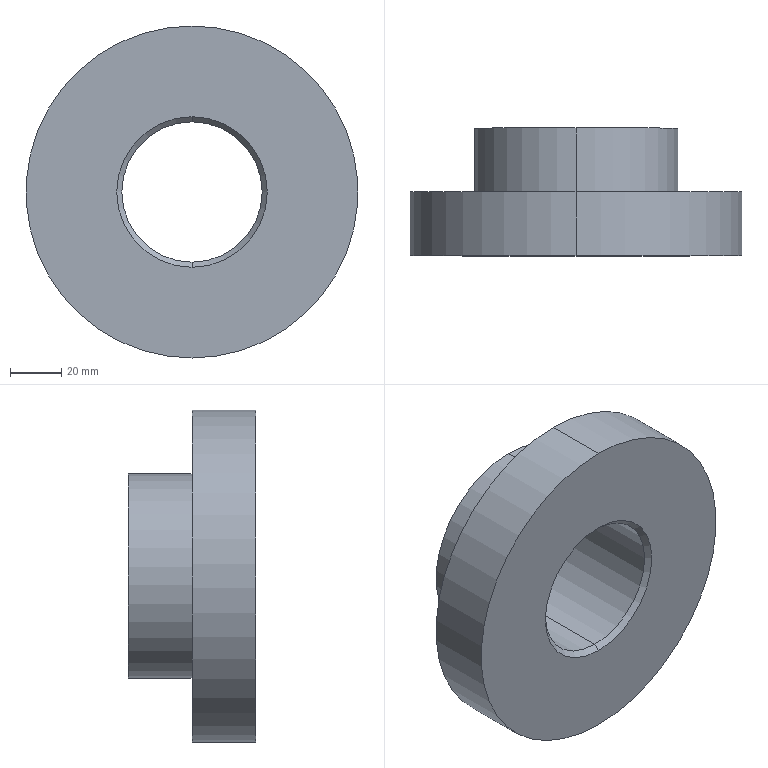Part | SolidWorks | features Revolution 1 | 1 solid | 11 faces | box 130 x 50 x 130 mm | volume 338349 mm3 | cylinder 6 | plane 3 | cone 2 | commonest cylinder face diameters 55 x2 80 x2 130 x2
STEP:
#1=CARTESIAN_POINT('',(0.,2.,27.5));
#2=VERTEX_POINT('',#1);
#3=CARTESIAN_POINT('',(0.,2.,-27.5));
#4=VERTEX_POINT('',#3);
#5=CARTESIAN_POINT('',(0.,2.,0.));
#6=DIRECTION('',(0.,-1.,0.));
#7=DIRECTION('',(0.,0.,-1.));
#8=AXIS2_PLACEMENT_3D('',#5,#6,#7);
#9=CIRCLE('',#8,27.5);
#10=EDGE_CURVE('',#2,#4,#9,.T.);
#11=ORIENTED_EDGE('',*,*,#10,.F.);
#12=CARTESIAN_POINT('',(0.,0.,29.5));
#13=VERTEX_POINT('',#12);
#14=CARTESIAN_POINT('',(0.,0.,29.5));
#15=DIRECTION('',(0.,-0.7071,0.7071));
#16=VECTOR('',#15,1000.);
#17=LINE('',#14,#16);
#18=EDGE_CURVE('',#2,#13,#17,.T.);
#19=ORIENTED_EDGE('',*,*,#18,.T.);
#20=CARTESIAN_POINT('',(0.,0.,-29.5));
#21=VERTEX_POINT('',#20);
#22=CARTESIAN_POINT('',(0.,0.,0.));
#23=DIRECTION('',(0.,-1.,0.));
#24=DIRECTION('',(0.,0.,-1.));
#25=AXIS2_PLACEMENT_3D('',#22,#23,#24);
#26=CIRCLE('',#25,29.5);
#27=EDGE_CURVE('',#13,#21,#26,.T.);
#28=ORIENTED_EDGE('',*,*,#27,.T.);
#29=CARTESIAN_POINT('',(0.,0.,-29.5));
#30=DIRECTION('',(0.,-0.7071,-0.7071));
#31=VECTOR('',#30,1000.);
#32=LINE('',#29,#31);
#33=EDGE_CURVE('',#4,#21,#32,.T.);
#34=ORIENTED_EDGE('',*,*,#33,.F.);
#35=EDGE_LOOP('',(#11,#19,#28,#34));
#36=FACE_OUTER_BOUND('',#35,.T.);
#37=CARTESIAN_POINT('',(0.,0.,0.));
#38=DIRECTION('',(0.,-1.,0.));
#39=DIRECTION('',(0.,0.,-1.));
#40=AXIS2_PLACEMENT_3D('',#37,#38,#39);
#41=CONICAL_SURFACE('',#40,29.5,0.7854);
#42=ADVANCED_FACE('',(#36),#41,.F.);
#43=CARTESIAN_POINT('',(0.,50.,27.5));
#44=VERTEX_POINT('',#43);
#45=CARTESIAN_POINT('',(0.,50.,-27.5));
#46=VERTEX_POINT('',#45);
#47=CARTESIAN_POINT('',(0.,50.,0.));
#48=DIRECTION('',(0.,-1.,0.));
#49=DIRECTION('',(0.,0.,-1.));
#50=AXIS2_PLACEMENT_3D('',#47,#48,#49);
#51=CIRCLE('',#50,27.5);
#52=EDGE_CURVE('',#44,#46,#51,.T.);
#53=ORIENTED_EDGE('',*,*,#52,.F.);
#54=CARTESIAN_POINT('',(0.,0.,27.5));
#55=DIRECTION('',(0.,-1.,0.));
#56=VECTOR('',#55,1000.);
#57=LINE('',#54,#56);
#58=EDGE_CURVE('',#44,#2,#57,.T.);
#59=ORIENTED_EDGE('',*,*,#58,.T.);
#60=ORIENTED_EDGE('',*,*,#10,.T.);
#61=CARTESIAN_POINT('',(0.,0.,-27.5));
#62=DIRECTION('',(0.,-1.,0.));
#63=VECTOR('',#62,1000.);
#64=LINE('',#61,#63);
#65=EDGE_CURVE('',#46,#4,#64,.T.);
#66=ORIENTED_EDGE('',*,*,#65,.F.);
#67=EDGE_LOOP('',(#53,#59,#60,#66));
#68=FACE_OUTER_BOUND('',#67,.T.);
#69=CARTESIAN_POINT('',(0.,0.,0.));
#70=DIRECTION('',(0.,-1.,0.));
#71=DIRECTION('',(0.,0.,-1.));
#72=AXIS2_PLACEMENT_3D('',#69,#70,#71);
#73=CYLINDRICAL_SURFACE('',#72,27.5);
#74=ADVANCED_FACE('',(#68),#73,.F.);
#75=CARTESIAN_POINT('',(0.,50.,-40.));
#76=VERTEX_POINT('',#75);
#77=CARTESIAN_POINT('',(0.,50.,40.));
#78=VERTEX_POINT('',#77);
#79=CARTESIAN_POINT('',(0.,50.,0.));
#80=DIRECTION('',(0.,-1.,0.));
#81=DIRECTION('',(0.,0.,-1.));
#82=AXIS2_PLACEMENT_3D('',#79,#80,#81);
#83=CIRCLE('',#82,40.);
#84=EDGE_CURVE('',#76,#78,#83,.T.);
#85=ORIENTED_EDGE('',*,*,#84,.T.);
#86=CARTESIAN_POINT('',(0.,25.,40.));
#87=VERTEX_POINT('',#86);
#88=CARTESIAN_POINT('',(0.,0.,40.));
#89=DIRECTION('',(0.,-1.,0.));
#90=VECTOR('',#89,1000.);
#91=LINE('',#88,#90);
#92=EDGE_CURVE('',#78,#87,#91,.T.);
#93=ORIENTED_EDGE('',*,*,#92,.T.);
#94=CARTESIAN_POINT('',(0.,25.,-40.));
#95=VERTEX_POINT('',#94);
#96=CARTESIAN_POINT('',(0.,25.,0.));
#97=DIRECTION('',(0.,-1.,0.));
#98=DIRECTION('',(0.,0.,-1.));
#99=AXIS2_PLACEMENT_3D('',#96,#97,#98);
#100=CIRCLE('',#99,40.);
#101=EDGE_CURVE('',#95,#87,#100,.T.);
#102=ORIENTED_EDGE('',*,*,#101,.F.);
#103=CARTESIAN_POINT('',(0.,0.,-40.));
#104=DIRECTION('',(0.,-1.,0.));
#105=VECTOR('',#104,1000.);
#106=LINE('',#103,#105);
#107=EDGE_CURVE('',#76,#95,#106,.T.);
#108=ORIENTED_EDGE('',*,*,#107,.F.);
#109=EDGE_LOOP('',(#85,#93,#102,#108));
#110=FACE_OUTER_BOUND('',#109,.T.);
#111=CARTESIAN_POINT('',(0.,0.,0.));
#112=DIRECTION('',(0.,-1.,0.));
#113=DIRECTION('',(0.,0.,-1.));
#114=AXIS2_PLACEMENT_3D('',#111,#112,#113);
#115=CYLINDRICAL_SURFACE('',#114,40.);
#116=ADVANCED_FACE('',(#110),#115,.T.);
#117=CARTESIAN_POINT('',(0.,25.,-65.));
#118=VERTEX_POINT('',#117);
#119=CARTESIAN_POINT('',(0.,25.,65.));
#120=VERTEX_POINT('',#119);
#121=CARTESIAN_POINT('',(0.,25.,0.));
#122=DIRECTION('',(0.,-1.,0.));
#123=DIRECTION('',(0.,0.,-1.));
#124=AXIS2_PLACEMENT_3D('',#121,#122,#123);
#125=CIRCLE('',#124,65.);
#126=EDGE_CURVE('',#118,#120,#125,.T.);
#127=ORIENTED_EDGE('',*,*,#126,.T.);
#128=CARTESIAN_POINT('',(0.,0.,65.));
#129=VERTEX_POINT('',#128);
#130=CARTESIAN_POINT('',(0.,0.,65.));
#131=DIRECTION('',(0.,-1.,0.));
#132=VECTOR('',#131,1000.);
#133=LINE('',#130,#132);
#134=EDGE_CURVE('',#120,#129,#133,.T.);
#135=ORIENTED_EDGE('',*,*,#134,.T.);
#136=CARTESIAN_POINT('',(0.,0.,-65.));
#137=VERTEX_POINT('',#136);
#138=CARTESIAN_POINT('',(0.,0.,0.));
#139=DIRECTION('',(0.,-1.,0.));
#140=DIRECTION('',(0.,0.,-1.));
#141=AXIS2_PLACEMENT_3D('',#138,#139,#140);
#142=CIRCLE('',#141,65.);
#143=EDGE_CURVE('',#137,#129,#142,.T.);
#144=ORIENTED_EDGE('',*,*,#143,.F.);
#145=CARTESIAN_POINT('',(0.,0.,-65.));
#146=DIRECTION('',(0.,-1.,0.));
#147=VECTOR('',#146,1000.);
#148=LINE('',#145,#147);
#149=EDGE_CURVE('',#118,#137,#148,.T.);
#150=ORIENTED_EDGE('',*,*,#149,.F.);
#151=EDGE_LOOP('',(#127,#135,#144,#150));
#152=FACE_OUTER_BOUND('',#151,.T.);
#153=CARTESIAN_POINT('',(0.,0.,0.));
#154=DIRECTION('',(0.,-1.,0.));
#155=DIRECTION('',(0.,0.,-1.));
#156=AXIS2_PLACEMENT_3D('',#153,#154,#155);
#157=CYLINDRICAL_SURFACE('',#156,65.);
#158=ADVANCED_FACE('',(#152),#157,.T.);
#159=ORIENTED_EDGE('',*,*,#134,.F.);
#160=CARTESIAN_POINT('',(0.,25.,0.));
#161=DIRECTION('',(0.,-1.,0.));
#162=DIRECTION('',(0.,0.,-1.));
#163=AXIS2_PLACEMENT_3D('',#160,#161,#162);
#164=CIRCLE('',#163,65.);
#165=EDGE_CURVE('',#120,#118,#164,.T.);
#166=ORIENTED_EDGE('',*,*,#165,.T.);
#167=ORIENTED_EDGE('',*,*,#149,.T.);
#168=CARTESIAN_POINT('',(0.,0.,0.));
#169=DIRECTION('',(0.,-1.,0.));
#170=DIRECTION('',(0.,0.,-1.));
#171=AXIS2_PLACEMENT_3D('',#168,#169,#170);
#172=CIRCLE('',#171,65.);
#173=EDGE_CURVE('',#129,#137,#172,.T.);
#174=ORIENTED_EDGE('',*,*,#173,.F.);
#175=EDGE_LOOP('',(#159,#166,#167,#174));
#176=FACE_OUTER_BOUND('',#175,.T.);
#177=CARTESIAN_POINT('',(0.,0.,0.));
#178=DIRECTION('',(0.,-1.,0.));
#179=DIRECTION('',(0.,0.,-1.));
#180=AXIS2_PLACEMENT_3D('',#177,#178,#179);
#181=CYLINDRICAL_SURFACE('',#180,65.);
#182=ADVANCED_FACE('',(#176),#181,.T.);
#183=ORIENTED_EDGE('',*,*,#126,.F.);
#184=ORIENTED_EDGE('',*,*,#165,.F.);
#185=EDGE_LOOP('',(#183,#184));
#186=FACE_OUTER_BOUND('',#185,.T.);
#187=ORIENTED_EDGE('',*,*,#101,.T.);
#188=CARTESIAN_POINT('',(0.,25.,0.));
#189=DIRECTION('',(0.,-1.,0.));
#190=DIRECTION('',(0.,0.,-1.));
#191=AXIS2_PLACEMENT_3D('',#188,#189,#190);
#192=CIRCLE('',#191,40.);
#193=EDGE_CURVE('',#87,#95,#192,.T.);
#194=ORIENTED_EDGE('',*,*,#193,.T.);
#195=EDGE_LOOP('',(#187,#194));
#196=FACE_BOUND('',#195,.T.);
#197=CARTESIAN_POINT('',(-65.,25.,0.));
#198=DIRECTION('',(0.,-1.,0.));
#199=DIRECTION('',(0.,0.,-1.));
#200=AXIS2_PLACEMENT_3D('',#197,#198,#199);
#201=PLANE('',#200);
#202=ADVANCED_FACE('',(#186,#196),#201,.F.);
#203=ORIENTED_EDGE('',*,*,#92,.F.);
#204=CARTESIAN_POINT('',(0.,50.,0.));
#205=DIRECTION('',(0.,-1.,0.));
#206=DIRECTION('',(0.,0.,-1.));
#207=AXIS2_PLACEMENT_3D('',#204,#205,#206);
#208=CIRCLE('',#207,40.);
#209=EDGE_CURVE('',#78,#76,#208,.T.);
#210=ORIENTED_EDGE('',*,*,#209,.T.);
#211=ORIENTED_EDGE('',*,*,#107,.T.);
#212=ORIENTED_EDGE('',*,*,#193,.F.);
#213=EDGE_LOOP('',(#203,#210,#211,#212));
#214=FACE_OUTER_BOUND('',#213,.T.);
#215=CARTESIAN_POINT('',(0.,0.,0.));
#216=DIRECTION('',(0.,-1.,0.));
#217=DIRECTION('',(0.,0.,-1.));
#218=AXIS2_PLACEMENT_3D('',#215,#216,#217);
#219=CYLINDRICAL_SURFACE('',#218,40.);
#220=ADVANCED_FACE('',(#214),#219,.T.);
#221=ORIENTED_EDGE('',*,*,#84,.F.);
#222=ORIENTED_EDGE('',*,*,#209,.F.);
#223=EDGE_LOOP('',(#221,#222));
#224=FACE_OUTER_BOUND('',#223,.T.);
#225=CARTESIAN_POINT('',(0.,50.,0.));
#226=DIRECTION('',(0.,-1.,0.));
#227=DIRECTION('',(0.,0.,-1.));
#228=AXIS2_PLACEMENT_3D('',#225,#226,#227);
#229=CIRCLE('',#228,27.5);
#230=EDGE_CURVE('',#46,#44,#229,.T.);
#231=ORIENTED_EDGE('',*,*,#230,.T.);
#232=ORIENTED_EDGE('',*,*,#52,.T.);
#233=EDGE_LOOP('',(#231,#232));
#234=FACE_BOUND('',#233,.T.);
#235=CARTESIAN_POINT('',(-40.,50.,0.));
#236=DIRECTION('',(0.,-1.,0.));
#237=DIRECTION('',(0.,0.,-1.));
#238=AXIS2_PLACEMENT_3D('',#235,#236,#237);
#239=PLANE('',#238);
#240=ADVANCED_FACE('',(#224,#234),#239,.F.);
#241=ORIENTED_EDGE('',*,*,#58,.F.);
#242=ORIENTED_EDGE('',*,*,#230,.F.);
#243=ORIENTED_EDGE('',*,*,#65,.T.);
#244=CARTESIAN_POINT('',(0.,2.,0.));
#245=DIRECTION('',(0.,-1.,0.));
#246=DIRECTION('',(0.,0.,-1.));
#247=AXIS2_PLACEMENT_3D('',#244,#245,#246);
#248=CIRCLE('',#247,27.5);
#249=EDGE_CURVE('',#4,#2,#248,.T.);
#250=ORIENTED_EDGE('',*,*,#249,.T.);
#251=EDGE_LOOP('',(#241,#242,#243,#250));
#252=FACE_OUTER_BOUND('',#251,.T.);
#253=CARTESIAN_POINT('',(0.,0.,0.));
#254=DIRECTION('',(0.,-1.,0.));
#255=DIRECTION('',(0.,0.,-1.));
#256=AXIS2_PLACEMENT_3D('',#253,#254,#255);
#257=CYLINDRICAL_SURFACE('',#256,27.5);
#258=ADVANCED_FACE('',(#252),#257,.F.);
#259=ORIENTED_EDGE('',*,*,#18,.F.);
#260=ORIENTED_EDGE('',*,*,#249,.F.);
#261=ORIENTED_EDGE('',*,*,#33,.T.);
#262=CARTESIAN_POINT('',(0.,0.,0.));
#263=DIRECTION('',(0.,-1.,0.));
#264=DIRECTION('',(0.,0.,-1.));
#265=AXIS2_PLACEMENT_3D('',#262,#263,#264);
#266=CIRCLE('',#265,29.5);
#267=EDGE_CURVE('',#21,#13,#266,.T.);
#268=ORIENTED_EDGE('',*,*,#267,.T.);
#269=EDGE_LOOP('',(#259,#260,#261,#268));
#270=FACE_OUTER_BOUND('',#269,.T.);
#271=CARTESIAN_POINT('',(0.,0.,0.));
#272=DIRECTION('',(0.,-1.,0.));
#273=DIRECTION('',(0.,0.,-1.));
#274=AXIS2_PLACEMENT_3D('',#271,#272,#273);
#275=CONICAL_SURFACE('',#274,29.5,0.7854);
#276=ADVANCED_FACE('',(#270),#275,.F.);
#277=ORIENTED_EDGE('',*,*,#267,.F.);
#278=ORIENTED_EDGE('',*,*,#27,.F.);
#279=EDGE_LOOP('',(#277,#278));
#280=FACE_BOUND('',#279,.T.);
#281=ORIENTED_EDGE('',*,*,#143,.T.);
#282=ORIENTED_EDGE('',*,*,#173,.T.);
#283=EDGE_LOOP('',(#281,#282));
#284=FACE_OUTER_BOUND('',#283,.T.);
#285=CARTESIAN_POINT('',(-29.5,0.,0.));
#286=DIRECTION('',(0.,1.,0.));
#287=DIRECTION('',(0.,0.,1.));
#288=AXIS2_PLACEMENT_3D('',#285,#286,#287);
#289=PLANE('',#288);
#290=ADVANCED_FACE('',(#280,#284),#289,.F.);
#291=CLOSED_SHELL('',(#42,#74,#116,#158,#182,#202,#220,#240,#258,#276,#290));
#292=MANIFOLD_SOLID_BREP('',#291);
#293=CARTESIAN_POINT('',(0.,0.,0.));
#294=DIRECTION('',(0.,0.,1.));
#295=DIRECTION('',(1.,0.,0.));
#296=AXIS2_PLACEMENT_3D('',#293,#294,#295);
#297=(LENGTH_UNIT()NAMED_UNIT(*)SI_UNIT(.MILLI.,.METRE.));
#298=UNCERTAINTY_MEASURE_WITH_UNIT(LENGTH_MEASURE(0.00001),#297,'','');
#299=(NAMED_UNIT(*)PLANE_ANGLE_UNIT()SI_UNIT($,.RADIAN.));
#300=(NAMED_UNIT(*)SI_UNIT($,.STERADIAN.)SOLID_ANGLE_UNIT());
#301=(GEOMETRIC_REPRESENTATION_CONTEXT(3)GLOBAL_UNCERTAINTY_ASSIGNED_CONTEXT((#298))GLOBAL_UNIT_ASSIGNED_CONTEXT((#297,#299,#300))REPRESENTATION_CONTEXT('',''));
#302=ADVANCED_BREP_SHAPE_REPRESENTATION('',(#292,#296),#301);